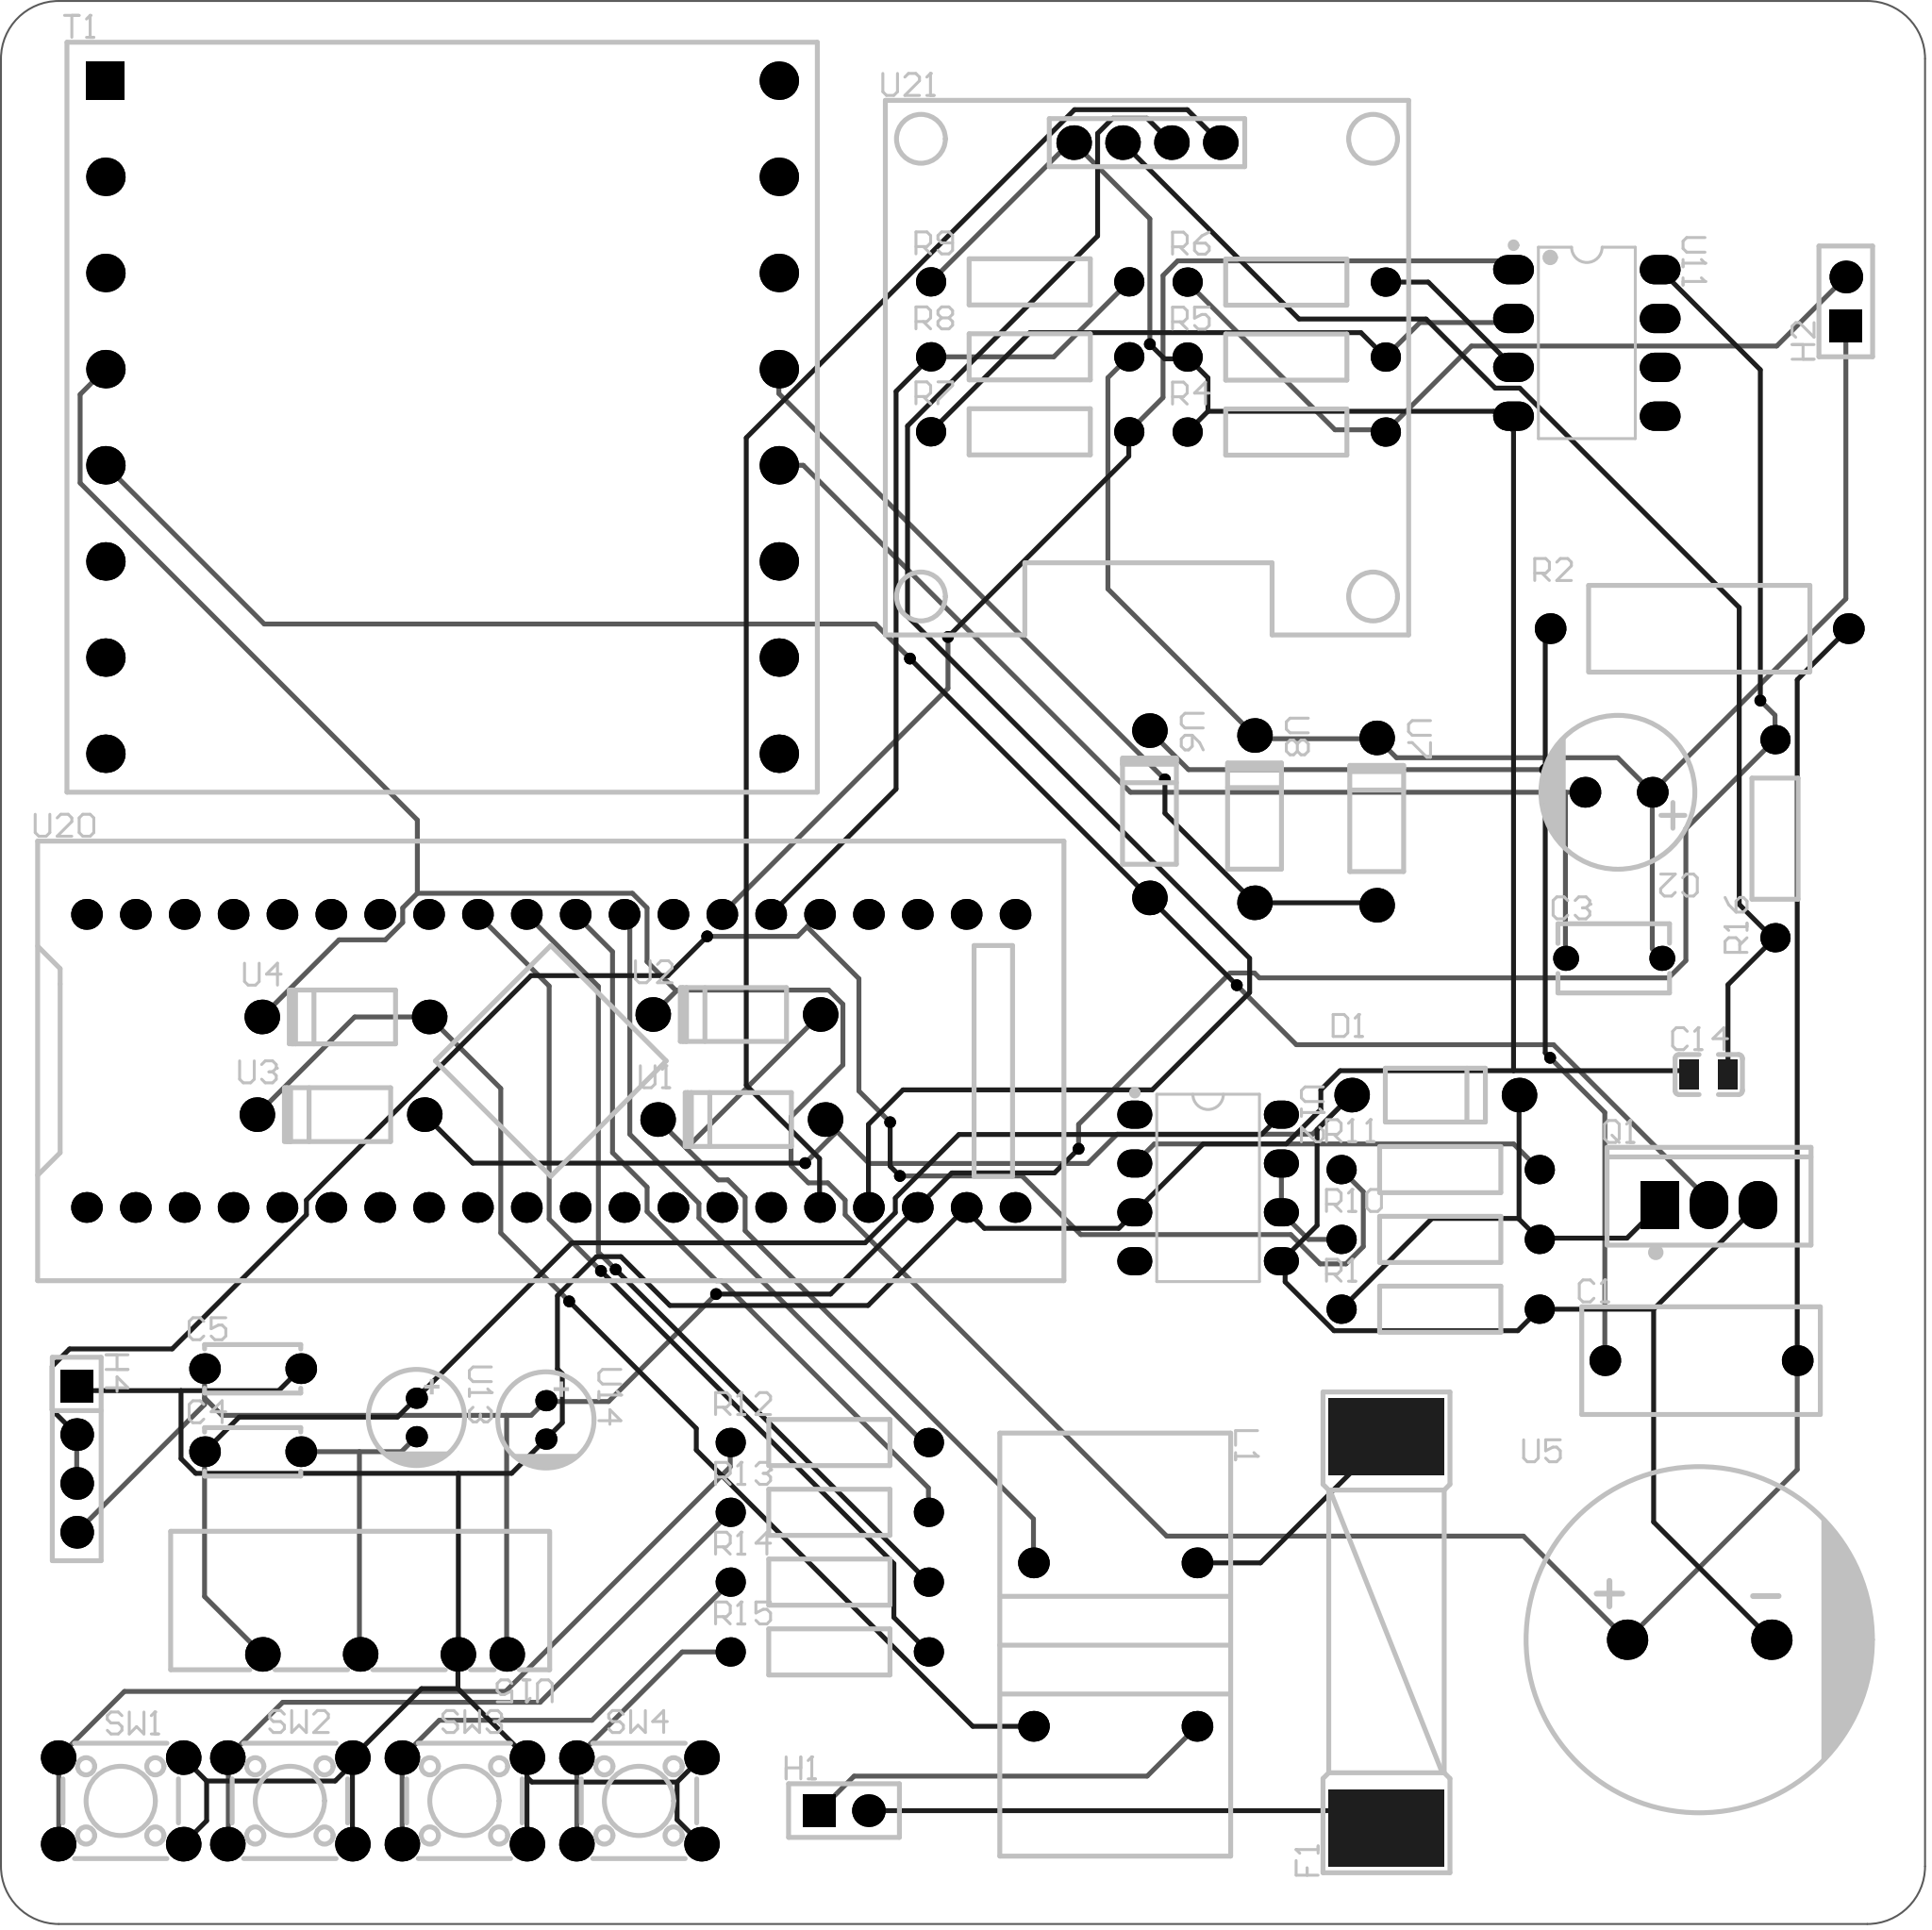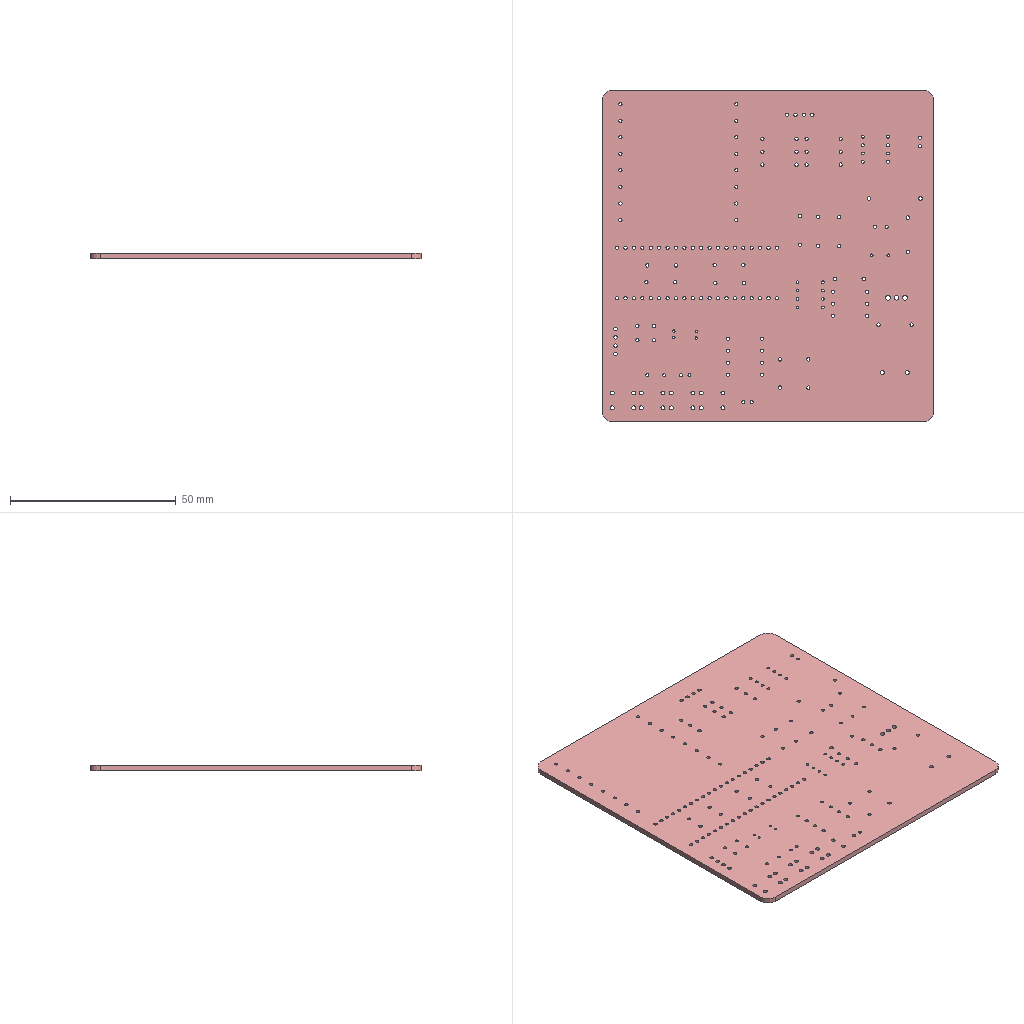Circuit board layout | Altium Designer | box 100 x 100 x 1.6 mm
Layer stack:
# Altium Designer layer stack of  (unit mm; dielectric type: 0 none, 1 core, 2 prepreg, 3 surface material)
index,name,kind,layer,copper_thickness_mm,dielectric_type,dielectric_thickness_mm,dielectric_material,dielectric_constant
0,Top Paste Mask Layer,other,,,,,,
1,Top Silkscreen Layer,other,,,,,,
2,Top Solder Mask Layer,dielectric,,,3,0.01,,3.3
3,Top Layer,copper,Top Layer,0.035,,,,
4,Dielectric1,dielectric,,,3,1.51,FR4,4.5
5,Bottom Layer,copper,Bottom Layer,0.035,,,,
6,Bottom Solder Mask Layer,dielectric,,,3,0.01,,3.3
7,Bottom Silkscreen Layer,other,,,,,,
8,Bottom Paste Mask Layer,other,,,,,,
# drill layer pairs: low layer,high layer
drill_pair,Top Layer,Bottom Layer
Part placement:
Designator,Comment,Layer,Footprint,Center-X(mm),Center-Y(mm),Rotation
C1,100uF,TopLayer,CAP-TH_L12.0-W5.5-P10.00-D1.0,164.557,105.496,0
C4,100nF,TopLayer,CAP-TH_L5.0-W2.5-P5.00-D1.0,89.281,100.762,0
C5,100nF,TopLayer,CAP-TH_L5.0-W2.5-P5.00-D1.0,89.281,105.08,0
D1,1N4742,TopLayer,DO-41_BD2.4-L4.7-P8.70-D0.8-FD,150.749,119.304,0
H1,,TopLayer,HDR-TH_2P-P2.54-V-F,120.015,82.093,0
H2,,TopLayer,HDR-TH_2P-P2.54-V-F,172.085,160.579,90
H4,,TopLayer,HDR-TH_4P-P2.54-V-F,80.137,100.381,270
L1,PDMCAT18107-103ML,TopLayer,IND-TH_4P-L22.0-W12.0-TR,134.112,90.729,270
Q1,FQPF8N60C,TopLayer,TO-220F-3_L10.2-W4.9-P2.54-L,164.973,113.589,0
R1,10kΩ,TopLayer,Res_1/4W,151.003,108.17,0
R2,10kΩ,TopLayer,Res_1W,164.465,143.561,0
C2,220uF,TopLayer,CAP-TH_BD8.0-P3.50-D0.6-FD,160.274,135.052,180
R5,2kΩ,TopLayer,Res_1/4W,143.002,157.683,0
R6,2kΩ,TopLayer,Res_1/4W,143.002,161.582,0
R7,200kΩ,TopLayer,Res_1/4W,129.667,153.797,0
R8,10kΩ,TopLayer,Res_1/4W,129.667,157.696,0
R9,2kΩ,TopLayer,Res_1/4W,129.667,161.595,0
R10,10Ω,TopLayer,Res_1/4W,151.003,111.8,0
R11,1kΩ,TopLayer,Res_1/4W,151.003,115.43,0
R12,2kΩ,TopLayer,Res_1/4W,119.253,101.238,0
R13,2kΩ,TopLayer,Res_1/4W,119.253,97.608,0
R14,2kΩ,TopLayer,Res_1/4W,119.253,93.978,0
R15,2kΩ,TopLayer,Res_1/4W,119.253,90.348,0
SW1,TS-1002-07026,TopLayer,SW-TH_4P-L6.0-W6.0-P4.50-LS6.5,82.423,82.601,0
SW2,TS-1002-07026,TopLayer,SW-TH_4P-L6.0-W6.0-P4.50-LS6.5,91.216,82.601,0
SW3,TS-1002-07026,TopLayer,SW-TH_4P-L6.0-W6.0-P4.50-LS6.5,100.288,82.601,0
SW4,TS-1002-07026,TopLayer,SW-TH_4P-L6.0-W6.0-P4.50-LS6.5,109.36,82.601,0
T1,,TopLayer,dip2_8_5mm_35MM,99.129,154.556,0
U1,1N4007,TopLayer,DO-41_BD2.4-L4.7-P8.70-D0.6-RD,114.681,118.034,0
U2,1N4007,TopLayer,DO-41_BD2.4-L4.7-P8.70-D0.6-RD,114.427,123.495,0
U3,1N4007,TopLayer,DO-41_BD2.4-L4.7-P8.70-D0.6-RD,93.853,118.288,0
U4,1N4007,TopLayer,DO-41_BD2.4-L4.7-P8.70-D0.6-RD,94.107,123.368,0
U5,150uF,TopLayer,CAP-TH_BD18.0-P7.50-D0.8-FD,164.465,90.983,0
U6,1N4007,TopLayer,DO-41_BD2.4-L4.7-P8.70-D0.6-RD,135.89,133.909,270
U11,LM358,TopLayer,DIP-8_L9.8-W6.4-P2.54-LS7.6-BL,158.623,158.42,270
U12,TLP250(F),TopLayer,DIP-8_L9.4-W6.4-P2.54-LS9.1-BL,138.938,114.478,270
U13,47uF,TopLayer,CAP-TH_BD5.0-P2.00-D0.5-FD,97.79,102.54,270
U14,100uF,TopLayer,CAP-TH_BD5.0-P2.00-D0.5-FD,104.521,102.413,270
U15,B0515S-2WR3,TopLayer,SIP-4_L19.5-W7.0-P2.54-L,96.139,90.221,180
R4,10mΩ,TopLayer,Res_1/4W,143.002,153.785,0
C3,1uF,TopLayer,CAP-TH_L5.8-W3.6-P5.0-D0.6,160.02,126.416,0
C14,100nF,TopLayer,C0805,164.958,120.374,0
F1,5F0.2R1,TopLayer,FUSE-SMD_5-20MM,148.209,91.364,90
R16,1kΩ,TopLayer,Res_1/4W,168.402,132.639,90
U7,1N4007,TopLayer,DO-41_BD2.4-L4.7-P8.70-D0.6-RD,147.701,133.528,270
U8,1N4007,TopLayer,DO-41_BD2.4-L4.7-P8.70-D0.6-RD,141.351,133.655,270
U20,LCKFB-DKX-STM32F103C8T6,TopLayer,CONN-TH_L53.3-W22.9_STM32F103C8T6-CARD,104.775,121.082,0
U21,HS96L03W2C03,TopLayer,OLED-TH_L27.8-W27.2-P2.54_C9900033791,135.763,168.834,0
Pad and via stacks:
# Altium Designer via and pad stacks of  (unit mm). Each distinct definition once, with the count of objects using it.
# via: kind,start_layer,end_layer,hole_mm,diameter_mm,mode(0 simple;1 top-mid-bottom;2 full stack),diameter_per_layer,count,example_net
# pad: kind,layer,hole_mm,hole_type(0 round;1 square;2 slot),plating,top_size,top_shape(1 round;2 rect;3 octagon;9 rounded rect),mid_size,bottom_size,mode,footprint,size_per_layer,count,example
pad,Multi-Layer,1,0,plated,1.6x1.6,1,1.6x1.6,1.6x1.6,0,CAP-TH_L12.0-W5.5-P10.00-D1.0,,2,C1.2
pad,Multi-Layer,1,0,plated,1.6x1.6,1,1.6x1.6,1.6x1.6,0,CAP-TH_L5.0-W2.5-P5.00-D1.0,,4,C4.1
pad,Multi-Layer,1.1,0,plated,1.8x1.8,1,1.8x1.8,1.8x1.8,0,DO-41_BD2.4-L4.7-P8.70-D0.8-FD,,2,D1.1
pad,Multi-Layer,1,0,plated,1.7x1.7,2,1.7x1.7,1.7x1.7,0,HDR-TH_2P-P2.54-V-F,,2,H1.1
pad,Multi-Layer,1,0,plated,1.7x1.7,1,1.7x1.7,1.7x1.7,0,HDR-TH_2P-P2.54-V-F,,2,H1.2
pad,Multi-Layer,1.1,0,plated,1.7x1.7,2,1.7x1.7,1.7x1.7,0,HDR-TH_4P-P2.54-V-F,,1,H4.1
pad,Multi-Layer,1.1,0,plated,1.7x1.7,1,1.7x1.7,1.7x1.7,0,HDR-TH_4P-P2.54-V-F,,3,H4.2
pad,Multi-Layer,1,0,plated,1.6x1.6,1,1.6x1.6,1.6x1.6,0,IND-TH_4P-L22.0-W12.0-TR,,4,L1.1
pad,Multi-Layer,1.4,0,plated,2x2.5,2,2x2.5,2x2.5,0,TO-220F-3_L10.2-W4.9-P2.54-L,,1,Q1.1
pad,Multi-Layer,1.4,0,plated,2x2.5,1,2x2.5,2x2.5,0,TO-220F-3_L10.2-W4.9-P2.54-L,,2,Q1.3
pad,Multi-Layer,1,0,plated,1.524x1.524,1,1.524x1.524,1.524x1.524,0,Res_1/4W,,28,R1.1
pad,Multi-Layer,1.1,0,plated,1.6x1.6,1,1.6x1.6,1.6x1.6,0,Res_1W,,2,R2.1
pad,Multi-Layer,1,0,plated,1.6x1.6,1,1.6x1.6,1.6x1.6,0,CAP-TH_BD8.0-P3.50-D0.6-FD,,2,C2.2
pad,Multi-Layer,1.2,0,plated,1.8x1.8,1,1.8x1.8,1.8x1.8,0,SW-TH_4P-L6.0-W6.0-P4.50-LS6.5,,16,SW1.1
pad,Multi-Layer,1,0,plated,2x2,2,2x2,2x2,0,dip2_8_5mm_35MM,,1,T1.1
pad,Multi-Layer,1,0,plated,2x2,1,2x2,2x2,0,dip2_8_5mm_35MM,,15,T1.2
pad,Multi-Layer,1,0,plated,1.8x1.8,1,1.8x1.8,1.8x1.8,0,DO-41_BD2.4-L4.7-P8.70-D0.6-RD,,14,U1.2
pad,Multi-Layer,1.2,0,plated,2.1x2.1,1,2.1x2.1,2.1x2.1,0,CAP-TH_BD18.0-P7.50-D0.8-FD,,2,U5.1
pad,Multi-Layer,0.9,0,plated,1.524x2.125,1,1.524x2.125,1.524x2.125,0,DIP-8_L9.8-W6.4-P2.54-LS7.6-BL,,8,U11.1
pad,Multi-Layer,0.8,0,plated,1.46x1.825,1,1.46x1.825,1.46x1.825,0,DIP-8_L9.4-W6.4-P2.54-LS9.1-BL,,8,U12.1
pad,Multi-Layer,0.7,0,plated,1.1x1.1,1,1.1x1.1,1.1x1.1,0,CAP-TH_BD5.0-P2.00-D0.5-FD,,4,U13.1
pad,Multi-Layer,0.9,0,plated,1.8x1.8,1,1.8x1.8,1.8x1.8,0,SIP-4_L19.5-W7.0-P2.54-L,,4,U15.1
pad,Multi-Layer,0.8,0,plated,1.3x1.3,1,1.3x1.3,1.3x1.3,0,CAP-TH_L5.8-W3.6-P5.0-D0.6,,2,C3.1
pad,Multi-Layer,1,0,plated,1.6x1.6,1,1.6x1.6,1.6x1.6,0,CONN-TH_L53.3-W22.9_STM32F103C8T6-CARD,,40,U20.1
pad,Multi-Layer,1.05,0,plated,1.8x1.8,1,1.8x1.8,1.8x1.8,0,OLED-TH_L27.8-W27.2-P2.54_C9900033791,,4,U21.1
pad,Top Layer,0,0,plated,1x1.55,2,1x1.55,1x1.55,0,C0805,,2,C14.1
pad,Top Layer,0,0,plated,4x6,2,4x6,4x6,0,FUSE-SMD_5-20MM,,2,F1.1
via,Top Layer,Bottom Layer,0.3048,0.61,0,,17,$1N2605